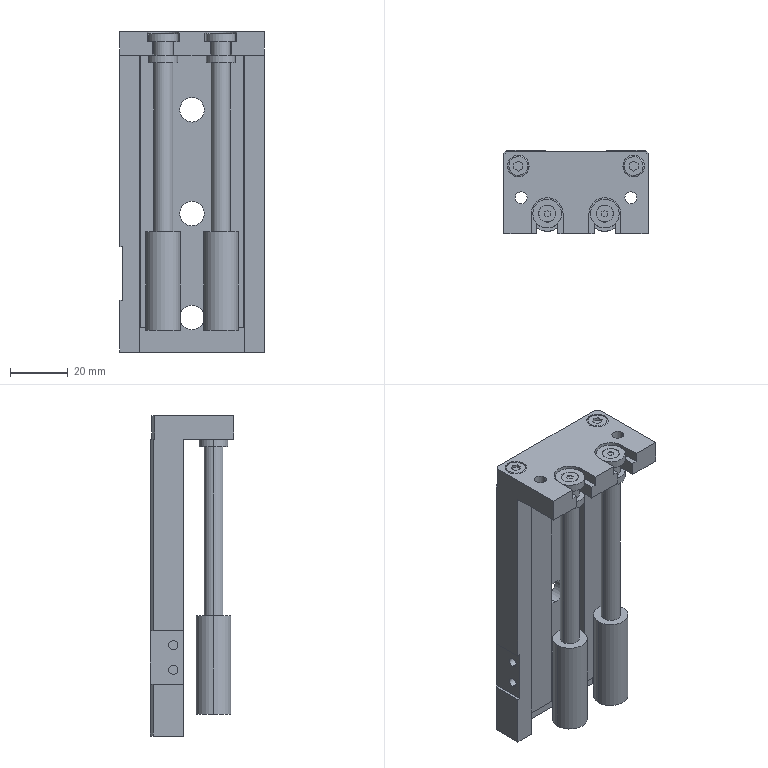Part | STEP file | QA-HI_MDX12x50-SD2BM2(0)_Ro | 1 solid | 182 faces | box 50 x 29 x 111 mm | volume 66088 mm3 | plane 111 | cylinder 67 | spline 4 | commonest cylinder face diameters 3.242 x16 6.7 x8 10 x8 7.5 x6 8.5 x6 4 x5